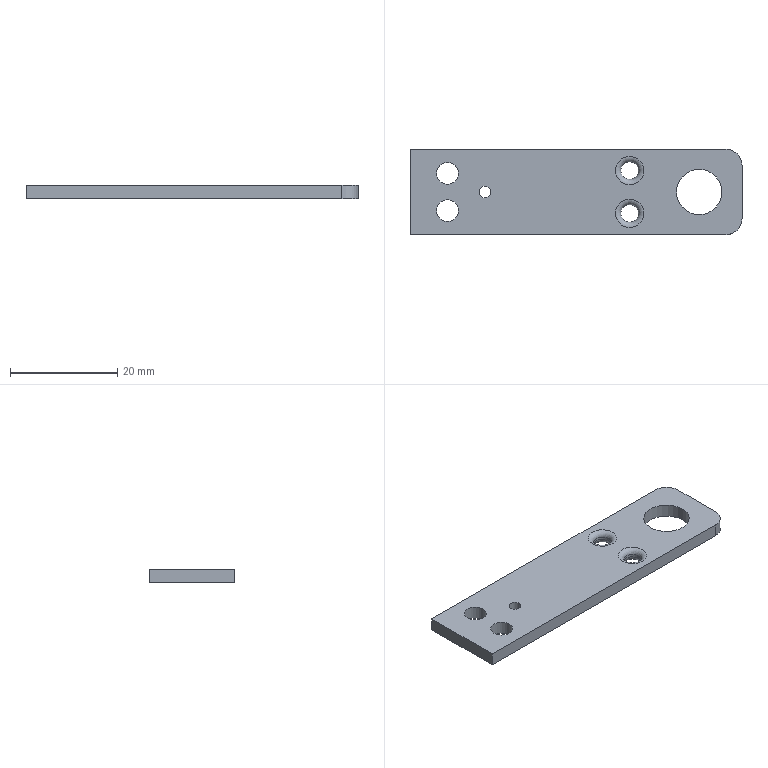Part | NX | features BREP 1 | 1 solid | 18 faces | box 62.05 x 16 x 2.5 mm | volume 2202 mm3 | cylinder 8 | plane 6 | torus 4 | commonest cylinder face diameters 3.3 x2 4.1 x2 6 x2 2.2 x1 8.5 x1
STEP:
#1=CARTESIAN_POINT('',(22.941,-1.063,1.));
#2=VERTEX_POINT('',#1);
#3=CARTESIAN_POINT('',(24.591,-1.063,1.));
#4=DIRECTION('',(0.,0.,1.));
#5=DIRECTION('',(-1.,0.,0.));
#6=AXIS2_PLACEMENT_3D('',#3,#4,#5);
#7=CIRCLE('',#6,1.65);
#8=EDGE_CURVE('',#2,#2,#7,.T.);
#9=ORIENTED_EDGE('',*,*,#8,.T.);
#10=EDGE_LOOP('',(#9));
#11=FACE_BOUND('',#10,.T.);
#12=CARTESIAN_POINT('',(21.941,-1.063,0.));
#13=VERTEX_POINT('',#12);
#14=CARTESIAN_POINT('',(24.591,-1.063,0.));
#15=DIRECTION('',(0.,0.,-1.));
#16=DIRECTION('',(-1.,0.,0.));
#17=AXIS2_PLACEMENT_3D('',#14,#15,#16);
#18=CIRCLE('',#17,2.65);
#19=EDGE_CURVE('',#13,#13,#18,.T.);
#20=ORIENTED_EDGE('',*,*,#19,.T.);
#21=EDGE_LOOP('',(#20));
#22=FACE_BOUND('',#21,.T.);
#23=CARTESIAN_POINT('',(24.591,-1.063,1.));
#24=DIRECTION('',(0.,0.,1.));
#25=DIRECTION('',(1.,0.,0.));
#26=AXIS2_PLACEMENT_3D('',#23,#24,#25);
#27=TOROIDAL_SURFACE('',#26,2.65,1.);
#28=ADVANCED_FACE('',(#11,#22),#27,.T.);
#29=CARTESIAN_POINT('',(-16.459,-5.063,0.));
#30=VERTEX_POINT('',#29);
#31=CARTESIAN_POINT('',(-16.459,10.937,0.));
#32=VERTEX_POINT('',#31);
#33=CARTESIAN_POINT('',(-16.459,-5.063,0.));
#34=DIRECTION('',(0.,1.,0.));
#35=VECTOR('',#34,1000.);
#36=LINE('',#33,#35);
#37=EDGE_CURVE('',#30,#32,#36,.T.);
#38=ORIENTED_EDGE('',*,*,#37,.T.);
#39=CARTESIAN_POINT('',(42.591,10.937,0.));
#40=VERTEX_POINT('',#39);
#41=CARTESIAN_POINT('',(-16.459,10.937,0.));
#42=DIRECTION('',(1.,0.,0.));
#43=VECTOR('',#42,1000.);
#44=LINE('',#41,#43);
#45=EDGE_CURVE('',#32,#40,#44,.T.);
#46=ORIENTED_EDGE('',*,*,#45,.T.);
#47=CARTESIAN_POINT('',(45.591,7.937,0.));
#48=VERTEX_POINT('',#47);
#49=CARTESIAN_POINT('',(42.591,7.937,0.));
#50=DIRECTION('',(0.,0.,-1.));
#51=DIRECTION('',(-1.,0.,0.));
#52=AXIS2_PLACEMENT_3D('',#49,#50,#51);
#53=CIRCLE('',#52,3.);
#54=EDGE_CURVE('',#40,#48,#53,.T.);
#55=ORIENTED_EDGE('',*,*,#54,.T.);
#56=CARTESIAN_POINT('',(45.591,-2.063,0.));
#57=VERTEX_POINT('',#56);
#58=CARTESIAN_POINT('',(45.591,7.937,0.));
#59=DIRECTION('',(0.,-1.,0.));
#60=VECTOR('',#59,1000.);
#61=LINE('',#58,#60);
#62=EDGE_CURVE('',#48,#57,#61,.T.);
#63=ORIENTED_EDGE('',*,*,#62,.T.);
#64=CARTESIAN_POINT('',(42.591,-5.063,0.));
#65=VERTEX_POINT('',#64);
#66=CARTESIAN_POINT('',(42.591,-2.063,0.));
#67=DIRECTION('',(0.,0.,-1.));
#68=DIRECTION('',(0.,1.,0.));
#69=AXIS2_PLACEMENT_3D('',#66,#67,#68);
#70=CIRCLE('',#69,3.);
#71=EDGE_CURVE('',#57,#65,#70,.T.);
#72=ORIENTED_EDGE('',*,*,#71,.T.);
#73=CARTESIAN_POINT('',(42.591,-5.063,0.));
#74=DIRECTION('',(-1.,0.,0.));
#75=VECTOR('',#74,1000.);
#76=LINE('',#73,#75);
#77=EDGE_CURVE('',#65,#30,#76,.T.);
#78=ORIENTED_EDGE('',*,*,#77,.T.);
#79=EDGE_LOOP('',(#38,#46,#55,#63,#72,#78));
#80=FACE_BOUND('',#79,.T.);
#81=CARTESIAN_POINT('',(27.241,6.937,0.));
#82=VERTEX_POINT('',#81);
#83=CARTESIAN_POINT('',(24.591,6.937,0.));
#84=DIRECTION('',(0.,0.,-1.));
#85=DIRECTION('',(1.,0.,0.));
#86=AXIS2_PLACEMENT_3D('',#83,#84,#85);
#87=CIRCLE('',#86,2.65);
#88=EDGE_CURVE('',#82,#82,#87,.T.);
#89=ORIENTED_EDGE('',*,*,#88,.F.);
#90=EDGE_LOOP('',(#89));
#91=FACE_BOUND('',#90,.T.);
#92=CARTESIAN_POINT('',(33.341,2.937,0.));
#93=VERTEX_POINT('',#92);
#94=CARTESIAN_POINT('',(37.591,2.937,0.));
#95=DIRECTION('',(0.,0.,1.));
#96=DIRECTION('',(-1.,0.,0.));
#97=AXIS2_PLACEMENT_3D('',#94,#95,#96);
#98=CIRCLE('',#97,4.25);
#99=EDGE_CURVE('',#93,#93,#98,.T.);
#100=ORIENTED_EDGE('',*,*,#99,.T.);
#101=EDGE_LOOP('',(#100));
#102=FACE_BOUND('',#101,.T.);
#103=CARTESIAN_POINT('',(-11.509,-0.5626,0.));
#104=VERTEX_POINT('',#103);
#105=CARTESIAN_POINT('',(-9.459,-0.5626,0.));
#106=DIRECTION('',(0.,0.,1.));
#107=DIRECTION('',(-1.,0.,0.));
#108=AXIS2_PLACEMENT_3D('',#105,#106,#107);
#109=CIRCLE('',#108,2.05);
#110=EDGE_CURVE('',#104,#104,#109,.T.);
#111=ORIENTED_EDGE('',*,*,#110,.T.);
#112=EDGE_LOOP('',(#111));
#113=FACE_BOUND('',#112,.T.);
#114=CARTESIAN_POINT('',(-11.509,6.437,0.));
#115=VERTEX_POINT('',#114);
#116=CARTESIAN_POINT('',(-9.459,6.437,0.));
#117=DIRECTION('',(0.,0.,1.));
#118=DIRECTION('',(-1.,0.,0.));
#119=AXIS2_PLACEMENT_3D('',#116,#117,#118);
#120=CIRCLE('',#119,2.05);
#121=EDGE_CURVE('',#115,#115,#120,.T.);
#122=ORIENTED_EDGE('',*,*,#121,.T.);
#123=EDGE_LOOP('',(#122));
#124=FACE_BOUND('',#123,.T.);
#125=CARTESIAN_POINT('',(-3.559,2.937,0.));
#126=VERTEX_POINT('',#125);
#127=CARTESIAN_POINT('',(-2.459,2.937,0.));
#128=DIRECTION('',(0.,0.,1.));
#129=DIRECTION('',(-1.,0.,0.));
#130=AXIS2_PLACEMENT_3D('',#127,#128,#129);
#131=CIRCLE('',#130,1.1);
#132=EDGE_CURVE('',#126,#126,#131,.T.);
#133=ORIENTED_EDGE('',*,*,#132,.T.);
#134=EDGE_LOOP('',(#133));
#135=FACE_BOUND('',#134,.T.);
#136=ORIENTED_EDGE('',*,*,#19,.F.);
#137=EDGE_LOOP('',(#136));
#138=FACE_BOUND('',#137,.T.);
#139=CARTESIAN_POINT('',(14.034,2.937,0.));
#140=DIRECTION('',(0.,0.,1.));
#141=DIRECTION('',(1.,0.,0.));
#142=AXIS2_PLACEMENT_3D('',#139,#140,#141);
#143=PLANE('',#142);
#144=ADVANCED_FACE('',(#80,#91,#102,#113,#124,#135,#138),#143,.F.);
#145=CARTESIAN_POINT('',(22.941,-1.063,1.5));
#146=VERTEX_POINT('',#145);
#147=CARTESIAN_POINT('',(24.591,-1.063,1.5));
#148=DIRECTION('',(0.,0.,-1.));
#149=DIRECTION('',(-1.,0.,0.));
#150=AXIS2_PLACEMENT_3D('',#147,#148,#149);
#151=CIRCLE('',#150,1.65);
#152=EDGE_CURVE('',#146,#146,#151,.T.);
#153=ORIENTED_EDGE('',*,*,#152,.F.);
#154=EDGE_LOOP('',(#153));
#155=FACE_BOUND('',#154,.T.);
#156=ORIENTED_EDGE('',*,*,#8,.F.);
#157=EDGE_LOOP('',(#156));
#158=FACE_BOUND('',#157,.T.);
#159=CARTESIAN_POINT('',(24.591,-1.063,0.));
#160=DIRECTION('',(0.,0.,1.));
#161=DIRECTION('',(-1.,0.,0.));
#162=AXIS2_PLACEMENT_3D('',#159,#160,#161);
#163=CYLINDRICAL_SURFACE('',#162,1.65);
#164=ADVANCED_FACE('',(#155,#158),#163,.F.);
#165=CARTESIAN_POINT('',(26.241,6.937,1.));
#166=VERTEX_POINT('',#165);
#167=CARTESIAN_POINT('',(24.591,6.937,1.));
#168=DIRECTION('',(0.,0.,1.));
#169=DIRECTION('',(1.,0.,0.));
#170=AXIS2_PLACEMENT_3D('',#167,#168,#169);
#171=CIRCLE('',#170,1.65);
#172=EDGE_CURVE('',#166,#166,#171,.T.);
#173=ORIENTED_EDGE('',*,*,#172,.T.);
#174=EDGE_LOOP('',(#173));
#175=FACE_BOUND('',#174,.T.);
#176=ORIENTED_EDGE('',*,*,#88,.T.);
#177=EDGE_LOOP('',(#176));
#178=FACE_BOUND('',#177,.T.);
#179=CARTESIAN_POINT('',(24.591,6.937,1.));
#180=DIRECTION('',(0.,0.,1.));
#181=DIRECTION('',(1.,0.,0.));
#182=AXIS2_PLACEMENT_3D('',#179,#180,#181);
#183=TOROIDAL_SURFACE('',#182,2.65,1.);
#184=ADVANCED_FACE('',(#175,#178),#183,.T.);
#185=CARTESIAN_POINT('',(22.941,6.937,1.5));
#186=VERTEX_POINT('',#185);
#187=CARTESIAN_POINT('',(24.591,6.937,1.5));
#188=DIRECTION('',(0.,0.,-1.));
#189=DIRECTION('',(-1.,0.,0.));
#190=AXIS2_PLACEMENT_3D('',#187,#188,#189);
#191=CIRCLE('',#190,1.65);
#192=EDGE_CURVE('',#186,#186,#191,.T.);
#193=ORIENTED_EDGE('',*,*,#192,.F.);
#194=EDGE_LOOP('',(#193));
#195=FACE_BOUND('',#194,.T.);
#196=ORIENTED_EDGE('',*,*,#172,.F.);
#197=EDGE_LOOP('',(#196));
#198=FACE_BOUND('',#197,.T.);
#199=CARTESIAN_POINT('',(24.591,6.937,0.));
#200=DIRECTION('',(0.,0.,1.));
#201=DIRECTION('',(-1.,0.,0.));
#202=AXIS2_PLACEMENT_3D('',#199,#200,#201);
#203=CYLINDRICAL_SURFACE('',#202,1.65);
#204=ADVANCED_FACE('',(#195,#198),#203,.F.);
#205=ORIENTED_EDGE('',*,*,#152,.T.);
#206=EDGE_LOOP('',(#205));
#207=FACE_BOUND('',#206,.T.);
#208=CARTESIAN_POINT('',(21.941,-1.063,2.5));
#209=VERTEX_POINT('',#208);
#210=CARTESIAN_POINT('',(24.591,-1.063,2.5));
#211=DIRECTION('',(0.,0.,1.));
#212=DIRECTION('',(-1.,0.,0.));
#213=AXIS2_PLACEMENT_3D('',#210,#211,#212);
#214=CIRCLE('',#213,2.65);
#215=EDGE_CURVE('',#209,#209,#214,.T.);
#216=ORIENTED_EDGE('',*,*,#215,.T.);
#217=EDGE_LOOP('',(#216));
#218=FACE_BOUND('',#217,.T.);
#219=CARTESIAN_POINT('',(24.591,-1.063,1.5));
#220=DIRECTION('',(0.,0.,-1.));
#221=DIRECTION('',(-1.,0.,0.));
#222=AXIS2_PLACEMENT_3D('',#219,#220,#221);
#223=TOROIDAL_SURFACE('',#222,2.65,1.);
#224=ADVANCED_FACE('',(#207,#218),#223,.T.);
#225=CARTESIAN_POINT('',(-16.459,10.937,2.5));
#226=VERTEX_POINT('',#225);
#227=CARTESIAN_POINT('',(42.591,10.937,2.5));
#228=VERTEX_POINT('',#227);
#229=CARTESIAN_POINT('',(-16.459,10.937,2.5));
#230=DIRECTION('',(1.,0.,0.));
#231=VECTOR('',#230,1000.);
#232=LINE('',#229,#231);
#233=EDGE_CURVE('',#226,#228,#232,.T.);
#234=ORIENTED_EDGE('',*,*,#233,.F.);
#235=CARTESIAN_POINT('',(-16.459,-5.063,2.5));
#236=VERTEX_POINT('',#235);
#237=CARTESIAN_POINT('',(-16.459,-5.063,2.5));
#238=DIRECTION('',(0.,1.,0.));
#239=VECTOR('',#238,1000.);
#240=LINE('',#237,#239);
#241=EDGE_CURVE('',#236,#226,#240,.T.);
#242=ORIENTED_EDGE('',*,*,#241,.F.);
#243=CARTESIAN_POINT('',(42.591,-5.063,2.5));
#244=VERTEX_POINT('',#243);
#245=CARTESIAN_POINT('',(42.591,-5.063,2.5));
#246=DIRECTION('',(-1.,0.,0.));
#247=VECTOR('',#246,1000.);
#248=LINE('',#245,#247);
#249=EDGE_CURVE('',#244,#236,#248,.T.);
#250=ORIENTED_EDGE('',*,*,#249,.F.);
#251=CARTESIAN_POINT('',(45.591,-2.063,2.5));
#252=VERTEX_POINT('',#251);
#253=CARTESIAN_POINT('',(42.591,-2.063,2.5));
#254=DIRECTION('',(0.,0.,-1.));
#255=DIRECTION('',(0.,1.,0.));
#256=AXIS2_PLACEMENT_3D('',#253,#254,#255);
#257=CIRCLE('',#256,3.);
#258=EDGE_CURVE('',#252,#244,#257,.T.);
#259=ORIENTED_EDGE('',*,*,#258,.F.);
#260=CARTESIAN_POINT('',(45.591,7.937,2.5));
#261=VERTEX_POINT('',#260);
#262=CARTESIAN_POINT('',(45.591,7.937,2.5));
#263=DIRECTION('',(0.,-1.,0.));
#264=VECTOR('',#263,1000.);
#265=LINE('',#262,#264);
#266=EDGE_CURVE('',#261,#252,#265,.T.);
#267=ORIENTED_EDGE('',*,*,#266,.F.);
#268=CARTESIAN_POINT('',(42.591,7.937,2.5));
#269=DIRECTION('',(0.,0.,-1.));
#270=DIRECTION('',(-1.,0.,0.));
#271=AXIS2_PLACEMENT_3D('',#268,#269,#270);
#272=CIRCLE('',#271,3.);
#273=EDGE_CURVE('',#228,#261,#272,.T.);
#274=ORIENTED_EDGE('',*,*,#273,.F.);
#275=EDGE_LOOP('',(#234,#242,#250,#259,#267,#274));
#276=FACE_BOUND('',#275,.T.);
#277=CARTESIAN_POINT('',(21.941,6.937,2.5));
#278=VERTEX_POINT('',#277);
#279=CARTESIAN_POINT('',(24.591,6.937,2.5));
#280=DIRECTION('',(0.,0.,1.));
#281=DIRECTION('',(-1.,0.,0.));
#282=AXIS2_PLACEMENT_3D('',#279,#280,#281);
#283=CIRCLE('',#282,2.65);
#284=EDGE_CURVE('',#278,#278,#283,.T.);
#285=ORIENTED_EDGE('',*,*,#284,.F.);
#286=EDGE_LOOP('',(#285));
#287=FACE_BOUND('',#286,.T.);
#288=CARTESIAN_POINT('',(33.341,2.937,2.5));
#289=VERTEX_POINT('',#288);
#290=CARTESIAN_POINT('',(37.591,2.937,2.5));
#291=DIRECTION('',(0.,0.,-1.));
#292=DIRECTION('',(-1.,0.,0.));
#293=AXIS2_PLACEMENT_3D('',#290,#291,#292);
#294=CIRCLE('',#293,4.25);
#295=EDGE_CURVE('',#289,#289,#294,.T.);
#296=ORIENTED_EDGE('',*,*,#295,.T.);
#297=EDGE_LOOP('',(#296));
#298=FACE_BOUND('',#297,.T.);
#299=CARTESIAN_POINT('',(-11.509,-0.5626,2.5));
#300=VERTEX_POINT('',#299);
#301=CARTESIAN_POINT('',(-9.459,-0.5626,2.5));
#302=DIRECTION('',(0.,0.,-1.));
#303=DIRECTION('',(-1.,0.,0.));
#304=AXIS2_PLACEMENT_3D('',#301,#302,#303);
#305=CIRCLE('',#304,2.05);
#306=EDGE_CURVE('',#300,#300,#305,.T.);
#307=ORIENTED_EDGE('',*,*,#306,.T.);
#308=EDGE_LOOP('',(#307));
#309=FACE_BOUND('',#308,.T.);
#310=CARTESIAN_POINT('',(-11.509,6.437,2.5));
#311=VERTEX_POINT('',#310);
#312=CARTESIAN_POINT('',(-9.459,6.437,2.5));
#313=DIRECTION('',(0.,0.,-1.));
#314=DIRECTION('',(-1.,0.,0.));
#315=AXIS2_PLACEMENT_3D('',#312,#313,#314);
#316=CIRCLE('',#315,2.05);
#317=EDGE_CURVE('',#311,#311,#316,.T.);
#318=ORIENTED_EDGE('',*,*,#317,.T.);
#319=EDGE_LOOP('',(#318));
#320=FACE_BOUND('',#319,.T.);
#321=CARTESIAN_POINT('',(-3.559,2.937,2.5));
#322=VERTEX_POINT('',#321);
#323=CARTESIAN_POINT('',(-2.459,2.937,2.5));
#324=DIRECTION('',(0.,0.,-1.));
#325=DIRECTION('',(-1.,0.,0.));
#326=AXIS2_PLACEMENT_3D('',#323,#324,#325);
#327=CIRCLE('',#326,1.1);
#328=EDGE_CURVE('',#322,#322,#327,.T.);
#329=ORIENTED_EDGE('',*,*,#328,.T.);
#330=EDGE_LOOP('',(#329));
#331=FACE_BOUND('',#330,.T.);
#332=ORIENTED_EDGE('',*,*,#215,.F.);
#333=EDGE_LOOP('',(#332));
#334=FACE_BOUND('',#333,.T.);
#335=CARTESIAN_POINT('',(14.034,2.937,2.5));
#336=DIRECTION('',(0.,0.,1.));
#337=DIRECTION('',(1.,0.,0.));
#338=AXIS2_PLACEMENT_3D('',#335,#336,#337);
#339=PLANE('',#338);
#340=ADVANCED_FACE('',(#276,#287,#298,#309,#320,#331,#334),#339,.T.);
#341=ORIENTED_EDGE('',*,*,#192,.T.);
#342=EDGE_LOOP('',(#341));
#343=FACE_BOUND('',#342,.T.);
#344=ORIENTED_EDGE('',*,*,#284,.T.);
#345=EDGE_LOOP('',(#344));
#346=FACE_BOUND('',#345,.T.);
#347=CARTESIAN_POINT('',(24.591,6.937,1.5));
#348=DIRECTION('',(0.,0.,-1.));
#349=DIRECTION('',(-1.,0.,0.));
#350=AXIS2_PLACEMENT_3D('',#347,#348,#349);
#351=TOROIDAL_SURFACE('',#350,2.65,1.);
#352=ADVANCED_FACE('',(#343,#346),#351,.T.);
#353=ORIENTED_EDGE('',*,*,#295,.F.);
#354=EDGE_LOOP('',(#353));
#355=FACE_BOUND('',#354,.T.);
#356=ORIENTED_EDGE('',*,*,#99,.F.);
#357=EDGE_LOOP('',(#356));
#358=FACE_BOUND('',#357,.T.);
#359=CARTESIAN_POINT('',(37.591,2.937,0.));
#360=DIRECTION('',(0.,0.,1.));
#361=DIRECTION('',(-1.,0.,0.));
#362=AXIS2_PLACEMENT_3D('',#359,#360,#361);
#363=CYLINDRICAL_SURFACE('',#362,4.25);
#364=ADVANCED_FACE('',(#355,#358),#363,.F.);
#365=ORIENTED_EDGE('',*,*,#306,.F.);
#366=EDGE_LOOP('',(#365));
#367=FACE_BOUND('',#366,.T.);
#368=ORIENTED_EDGE('',*,*,#110,.F.);
#369=EDGE_LOOP('',(#368));
#370=FACE_BOUND('',#369,.T.);
#371=CARTESIAN_POINT('',(-9.459,-0.5626,0.));
#372=DIRECTION('',(0.,0.,1.));
#373=DIRECTION('',(-1.,0.,0.));
#374=AXIS2_PLACEMENT_3D('',#371,#372,#373);
#375=CYLINDRICAL_SURFACE('',#374,2.05);
#376=ADVANCED_FACE('',(#367,#370),#375,.F.);
#377=ORIENTED_EDGE('',*,*,#317,.F.);
#378=EDGE_LOOP('',(#377));
#379=FACE_BOUND('',#378,.T.);
#380=ORIENTED_EDGE('',*,*,#121,.F.);
#381=EDGE_LOOP('',(#380));
#382=FACE_BOUND('',#381,.T.);
#383=CARTESIAN_POINT('',(-9.459,6.437,0.));
#384=DIRECTION('',(0.,0.,1.));
#385=DIRECTION('',(-1.,0.,0.));
#386=AXIS2_PLACEMENT_3D('',#383,#384,#385);
#387=CYLINDRICAL_SURFACE('',#386,2.05);
#388=ADVANCED_FACE('',(#379,#382),#387,.F.);
#389=ORIENTED_EDGE('',*,*,#328,.F.);
#390=EDGE_LOOP('',(#389));
#391=FACE_BOUND('',#390,.T.);
#392=ORIENTED_EDGE('',*,*,#132,.F.);
#393=EDGE_LOOP('',(#392));
#394=FACE_BOUND('',#393,.T.);
#395=CARTESIAN_POINT('',(-2.459,2.937,0.));
#396=DIRECTION('',(0.,0.,1.));
#397=DIRECTION('',(-1.,0.,0.));
#398=AXIS2_PLACEMENT_3D('',#395,#396,#397);
#399=CYLINDRICAL_SURFACE('',#398,1.1);
#400=ADVANCED_FACE('',(#391,#394),#399,.F.);
#401=ORIENTED_EDGE('',*,*,#233,.T.);
#402=CARTESIAN_POINT('',(42.591,10.937,0.));
#403=DIRECTION('',(0.,0.,1.));
#404=VECTOR('',#403,1000.);
#405=LINE('',#402,#404);
#406=EDGE_CURVE('',#40,#228,#405,.T.);
#407=ORIENTED_EDGE('',*,*,#406,.F.);
#408=ORIENTED_EDGE('',*,*,#45,.F.);
#409=CARTESIAN_POINT('',(-16.459,10.937,0.));
#410=DIRECTION('',(0.,0.,1.));
#411=VECTOR('',#410,1000.);
#412=LINE('',#409,#411);
#413=EDGE_CURVE('',#32,#226,#412,.T.);
#414=ORIENTED_EDGE('',*,*,#413,.T.);
#415=EDGE_LOOP('',(#401,#407,#408,#414));
#416=FACE_BOUND('',#415,.T.);
#417=CARTESIAN_POINT('',(-16.459,10.937,0.));
#418=DIRECTION('',(0.,1.,0.));
#419=DIRECTION('',(0.,0.,1.));
#420=AXIS2_PLACEMENT_3D('',#417,#418,#419);
#421=PLANE('',#420);
#422=ADVANCED_FACE('',(#416),#421,.T.);
#423=ORIENTED_EDGE('',*,*,#273,.T.);
#424=CARTESIAN_POINT('',(45.591,7.937,0.));
#425=DIRECTION('',(0.,0.,1.));
#426=VECTOR('',#425,1000.);
#427=LINE('',#424,#426);
#428=EDGE_CURVE('',#48,#261,#427,.T.);
#429=ORIENTED_EDGE('',*,*,#428,.F.);
#430=ORIENTED_EDGE('',*,*,#54,.F.);
#431=ORIENTED_EDGE('',*,*,#406,.T.);
#432=EDGE_LOOP('',(#423,#429,#430,#431));
#433=FACE_BOUND('',#432,.T.);
#434=CARTESIAN_POINT('',(42.591,7.937,0.));
#435=DIRECTION('',(0.,0.,1.));
#436=DIRECTION('',(-1.,0.,0.));
#437=AXIS2_PLACEMENT_3D('',#434,#435,#436);
#438=CYLINDRICAL_SURFACE('',#437,3.);
#439=ADVANCED_FACE('',(#433),#438,.T.);
#440=ORIENTED_EDGE('',*,*,#266,.T.);
#441=CARTESIAN_POINT('',(45.591,-2.063,0.));
#442=DIRECTION('',(0.,0.,1.));
#443=VECTOR('',#442,1000.);
#444=LINE('',#441,#443);
#445=EDGE_CURVE('',#57,#252,#444,.T.);
#446=ORIENTED_EDGE('',*,*,#445,.F.);
#447=ORIENTED_EDGE('',*,*,#62,.F.);
#448=ORIENTED_EDGE('',*,*,#428,.T.);
#449=EDGE_LOOP('',(#440,#446,#447,#448));
#450=FACE_BOUND('',#449,.T.);
#451=CARTESIAN_POINT('',(45.591,7.937,0.));
#452=DIRECTION('',(1.,0.,0.));
#453=DIRECTION('',(0.,0.,-1.));
#454=AXIS2_PLACEMENT_3D('',#451,#452,#453);
#455=PLANE('',#454);
#456=ADVANCED_FACE('',(#450),#455,.T.);
#457=ORIENTED_EDGE('',*,*,#258,.T.);
#458=CARTESIAN_POINT('',(42.591,-5.063,0.));
#459=DIRECTION('',(0.,0.,1.));
#460=VECTOR('',#459,1000.);
#461=LINE('',#458,#460);
#462=EDGE_CURVE('',#65,#244,#461,.T.);
#463=ORIENTED_EDGE('',*,*,#462,.F.);
#464=ORIENTED_EDGE('',*,*,#71,.F.);
#465=ORIENTED_EDGE('',*,*,#445,.T.);
#466=EDGE_LOOP('',(#457,#463,#464,#465));
#467=FACE_BOUND('',#466,.T.);
#468=CARTESIAN_POINT('',(42.591,-2.063,0.));
#469=DIRECTION('',(0.,0.,1.));
#470=DIRECTION('',(0.,1.,0.));
#471=AXIS2_PLACEMENT_3D('',#468,#469,#470);
#472=CYLINDRICAL_SURFACE('',#471,3.);
#473=ADVANCED_FACE('',(#467),#472,.T.);
#474=ORIENTED_EDGE('',*,*,#249,.T.);
#475=CARTESIAN_POINT('',(-16.459,-5.063,0.));
#476=DIRECTION('',(0.,0.,1.));
#477=VECTOR('',#476,1000.);
#478=LINE('',#475,#477);
#479=EDGE_CURVE('',#30,#236,#478,.T.);
#480=ORIENTED_EDGE('',*,*,#479,.F.);
#481=ORIENTED_EDGE('',*,*,#77,.F.);
#482=ORIENTED_EDGE('',*,*,#462,.T.);
#483=EDGE_LOOP('',(#474,#480,#481,#482));
#484=FACE_BOUND('',#483,.T.);
#485=CARTESIAN_POINT('',(42.591,-5.063,0.));
#486=DIRECTION('',(0.,-1.,0.));
#487=DIRECTION('',(0.,0.,-1.));
#488=AXIS2_PLACEMENT_3D('',#485,#486,#487);
#489=PLANE('',#488);
#490=ADVANCED_FACE('',(#484),#489,.T.);
#491=ORIENTED_EDGE('',*,*,#241,.T.);
#492=ORIENTED_EDGE('',*,*,#413,.F.);
#493=ORIENTED_EDGE('',*,*,#37,.F.);
#494=ORIENTED_EDGE('',*,*,#479,.T.);
#495=EDGE_LOOP('',(#491,#492,#493,#494));
#496=FACE_BOUND('',#495,.T.);
#497=CARTESIAN_POINT('',(-16.459,-5.063,0.));
#498=DIRECTION('',(-1.,0.,0.));
#499=DIRECTION('',(0.,0.,1.));
#500=AXIS2_PLACEMENT_3D('',#497,#498,#499);
#501=PLANE('',#500);
#502=ADVANCED_FACE('',(#496),#501,.T.);
#503=CLOSED_SHELL('',(#28,#144,#164,#184,#204,#224,#340,#352,#364,#376,#388,#400,#422,#439,#456,#473,#490,#502));
#504=MANIFOLD_SOLID_BREP('',#503);
#505=(LENGTH_UNIT()NAMED_UNIT(*)SI_UNIT(.MILLI.,.METRE.));
#506=UNCERTAINTY_MEASURE_WITH_UNIT(LENGTH_MEASURE(0.00001),#505,'','');
#507=(NAMED_UNIT(*)PLANE_ANGLE_UNIT()SI_UNIT($,.RADIAN.));
#508=(NAMED_UNIT(*)SI_UNIT($,.STERADIAN.)SOLID_ANGLE_UNIT());
#509=(GEOMETRIC_REPRESENTATION_CONTEXT(3)GLOBAL_UNCERTAINTY_ASSIGNED_CONTEXT((#506))GLOBAL_UNIT_ASSIGNED_CONTEXT((#505,#507,#508))REPRESENTATION_CONTEXT('',''));
#510=ADVANCED_BREP_SHAPE_REPRESENTATION('',(#504),#509);